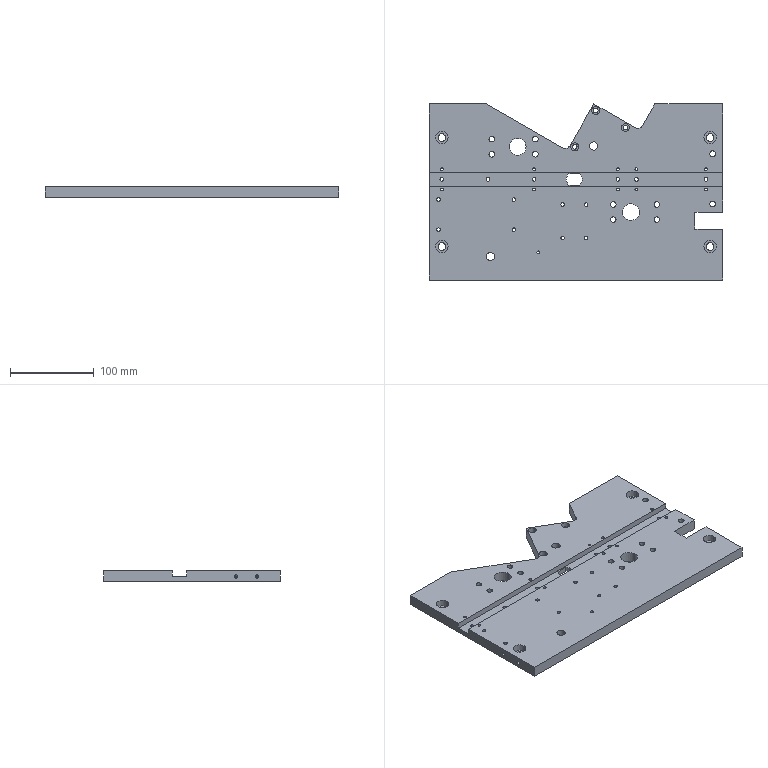Part | STEP file | middle plate | 1 solid | 171 faces | box 350 x 210 x 13 mm | volume 812608 mm3 | cylinder 131 | plane 36 | cone 4 | commonest cylinder face diameters 3.3 x22 4.2 x20 6.6 x16 11 x16 4.5 x12 9 x8